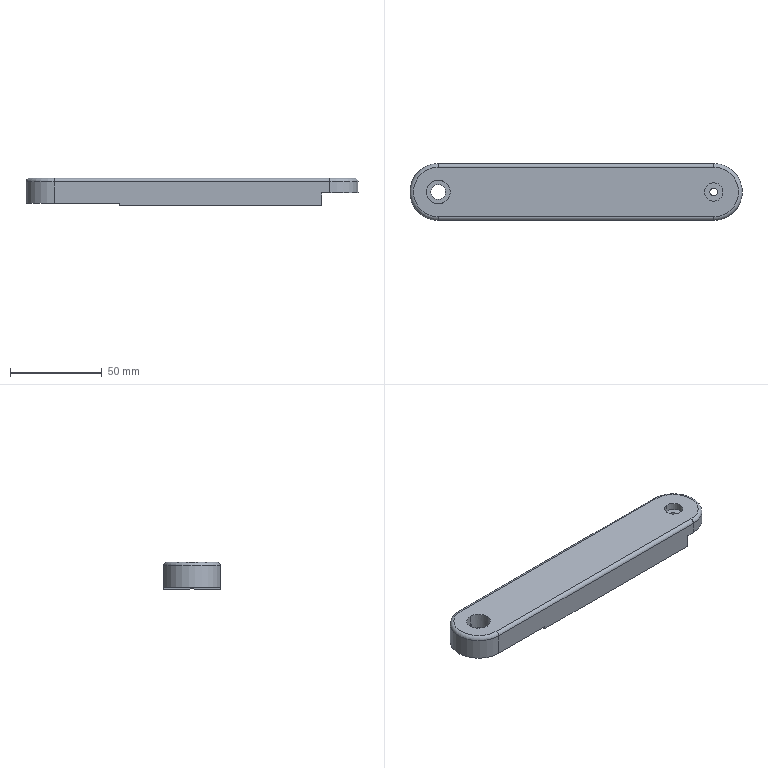NC program | NX | posted with a generic post | part box 181 x 31 x 15 mm
Lines 1657 to 2910 of 2910:
(FIXED_CONTOUR , TOOL : R2)
N3222 T21 M6
N3224 G54
N3226 G17 G0 G90 X1.241 Y-0.541 S9500 M3
N3228 G43 Z30. H21
N3230 Z3.6
N3232 G94 G1 Z-0.539 F1000.
N3234 X1.217 Y-0.511
N3236 X1.179 Y-0.512
N3238 X1.1 F2500.
N3240 X-0.1
N3242 X-1.3
N3244 X-2.5
N3246 X-3.7
N3248 X-4.9 Z-0.54
N3250 X-6.1 Y-0.511
N3252 X-7.3
N3254 X-8.5
N3256 X-9.7 Z-0.541
N3258 X-10.9
N3260 X-12.1
N3262 X-13.3 Z-0.542
N3264 X-14.5
N3266 X-15.7
N3268 X-16.9 Y-0.51 Z-0.543
N3270 X-18.1
N3272 X-19.3 Z-0.544
N3274 X-20.5
N3276 X-21.7 Z-0.545
N3278 X-22.9
N3280 X-24.1
N3282 X-25.3 Z-0.546
N3284 X-26.5 Y-0.509
N3286 X-27.7 Z-0.547
N3288 X-28.9
N3290 X-30.1 Z-0.548
N3292 X-31.3
N3294 X-32.5 Z-0.549
N3296 X-33.7
N3298 X-34.9
N3300 X-36.1 Y-0.508 Z-0.55
N3302 X-37.3
N3304 X-38.5
N3306 X-39.7
N3308 X-40.9
N3310 X-42.1
N3312 X-43.3
N3314 X-44.5 Z-0.551
N3316 X-45.7
N3318 X-46.9 Y-0.507
N3320 X-48.1
N3322 X-49.3
N3324 X-50.5
N3326 X-51.7
N3328 X-52.9
N3330 X-54.1
N3332 X-55.3 Z-0.552
N3334 X-56.5 Y-0.506
N3336 X-57.7
N3338 X-58.9
N3340 X-59.348
N3342 X-59.324 Y-0.42 Z-0.62
N3344 X-58.9
N3346 X-57.7 Z-0.619
N3348 X-56.5
N3350 X-55.3
N3352 X-54.1 Z-0.618
N3354 X-52.9 Y-0.421
N3356 X-51.7 Z-0.617
N3358 X-50.5
N3360 X-49.3 Z-0.616
N3362 X-48.1
N3364 X-46.9 Z-0.615
N3366 X-45.7
N3368 X-44.5
N3370 X-43.3 Y-0.422 Z-0.614
N3372 X-42.1
N3374 X-40.9 Z-0.613
N3376 X-39.7
N3378 X-38.5 Z-0.612
N3380 X-37.3
N3382 X-36.1
N3384 X-34.9 Z-0.611
N3386 X-33.7
N3388 X-32.5 Y-0.423
N3390 X-31.3
N3392 X-30.1 Z-0.61
N3394 X-28.9
N3396 X-27.7
N3398 X-26.5
N3400 X-25.3 Z-0.609
N3402 X-24.1
N3404 X-22.9 Y-0.424
N3406 X-21.7
N3408 X-20.5
N3410 X-19.3
N3412 X-18.1
N3414 X-16.9
N3416 X-15.7 Z-0.608
N3418 X-14.5
N3420 X-13.3
N3422 X-12.1 Y-0.425
N3424 X-10.9
N3426 X-9.7
N3428 X-8.5
N3430 X-7.3
N3432 X-6.1
N3434 X-4.9
N3436 X-3.7
N3438 X-2.5 Y-0.426 Z-0.607
N3440 X-1.3
N3442 X-0.1
N3444 X1.1
N3446 X2.3
N3448 X3.5
N3450 X4.7
N3452 X5.9
N3454 X7.1
N3456 X8.3 Y-0.427
N3458 X9.5
N3460 X10.7 Z-0.606
N3462 X11.9
N3464 X13.1
N3466 X14.3
N3468 X15.5
N3470 X16.7
N3472 X17.9 Y-0.428
N3474 X19.1
N3476 X20.3
N3478 X21.5
N3480 X22.7 Z-0.605
N3482 X23.9
N3484 X25.1
N3486 X26.3
N3488 X27.5 Y-0.429
N3490 X28.7
N3492 X29.9
N3494 X31.1
N3496 X32.3
N3498 X33.5
N3500 X34.7
N3502 X35.9 Z-0.604
N3504 X37.1
N3506 X38.3 Y-0.43
N3508 X39.5
N3510 Y-0.391 Z-0.63
N3512 Y-0.336 Z-0.66
N3514 X38.3 Y-0.335
N3516 X37.1
N3518 X35.9 Z-0.661
N3520 X34.7
N3522 X33.5
N3524 X32.3
N3526 X31.1
N3528 X29.9
N3530 X28.7
N3532 X27.5 Y-0.334
N3534 X26.3
N3536 X25.1
N3538 X23.9
N3540 X22.7
N3542 X21.5
N3544 X20.3
N3546 X19.1
N3548 X17.9 Y-0.333 Z-0.662
N3550 X16.7
N3552 X15.5
N3554 X14.3
N3556 X13.1
N3558 X11.9
N3560 X10.7
N3562 X9.5
N3564 X8.3 Y-0.332
N3566 X7.1
N3568 X5.9
N3570 X4.7
N3572 X3.5
N3574 X2.3
N3576 X1.1
N3578 X-0.1 Z-0.663
N3580 X-1.3
N3582 X-2.5 Y-0.331
N3584 X-3.7
N3586 X-4.9
N3588 X-6.1
N3590 X-7.3
N3592 X-8.5
N3594 X-9.7
N3596 X-10.9
N3598 X-12.1 Y-0.33
N3600 X-13.3
N3602 X-14.5
N3604 X-15.7
N3606 X-16.9
N3608 X-18.1
N3610 X-19.3 Z-0.664
N3612 X-20.5
N3614 X-21.7
N3616 X-22.9 Y-0.329
N3618 X-24.1
N3620 X-25.3
N3622 X-26.5 Z-0.665
N3624 X-27.7
N3626 X-28.9
N3628 X-30.1
N3630 X-31.3
N3632 X-32.5 Y-0.328 Z-0.666
N3634 X-33.7
N3636 X-34.9
N3638 X-36.1 Z-0.667
N3640 X-37.3
N3642 X-38.5
N3644 X-39.7 Z-0.668
N3646 X-40.9
N3648 X-42.1
N3650 X-43.3 Y-0.327 Z-0.669
N3652 X-44.5
N3654 X-45.7
N3656 X-46.9 Z-0.67
N3658 X-48.1
N3660 X-49.3
N3662 X-50.5 Z-0.671
N3664 X-51.7
N3666 X-52.9 Y-0.326
N3668 X-54.1
N3670 X-55.3 Z-0.672
N3672 X-56.5
N3674 X-57.7
N3676 X-58.9 Z-0.673
N3678 X-59.301
N3680 X-59.281 Y-0.232 Z-0.711
N3682 X-58.9
N3684 X-57.7
N3686 X-56.5 Z-0.71
N3688 X-55.3
N3690 X-54.1
N3692 X-52.9 Z-0.709
N3694 X-51.7
N3696 X-50.5 Y-0.233
N3698 X-49.3
N3700 X-48.1 Z-0.708
N3702 X-46.9
N3704 X-45.7
N3706 X-44.5 Z-0.707
N3708 X-43.3
N3710 X-42.1
N3712 X-40.9 Y-0.234
N3714 X-39.7 Z-0.706
N3716 X-38.5
N3718 X-37.3
N3720 X-36.1 Z-0.705
N3722 X-34.9
N3724 X-33.7
N3726 X-32.5
N3728 X-31.3 Z-0.704
N3730 X-30.1 Y-0.235
N3732 X-28.9
N3734 X-27.7
N3736 X-26.5 Z-0.703
N3738 X-25.3
N3740 X-24.1
N3742 X-22.9
N3744 X-21.7 Z-0.702
N3746 X-20.5 Y-0.236
N3748 X-19.3
N3750 X-18.1
N3752 X-16.9
N3754 X-15.7
N3756 X-14.5
N3758 X-13.3
N3760 X-12.1
N3762 X-10.9
N3764 X-9.7 Y-0.237
N3766 X-8.5 Z-0.701
N3768 X-7.3
N3770 X-6.1
N3772 X-4.9
N3774 X-3.7
N3776 X-2.5
N3778 X-1.3
N3780 X-0.1 Y-0.238
N3782 X1.1
N3784 X2.3
N3786 X3.5
N3788 X4.7
N3790 X5.9
N3792 X7.1
N3794 X8.3
N3796 X9.5
N3798 X10.7 Y-0.239
N3800 X11.9
N3802 X13.1
N3804 X14.3
N3806 X15.5
N3808 X16.7
N3810 X17.9
N3812 X19.1
N3814 X20.3 Y-0.24 Z-0.7
N3816 X21.5
N3818 X22.7
N3820 X23.9
N3822 X25.1
N3824 X26.3
N3826 X27.5
N3828 X28.7
N3830 X29.9 Y-0.241
N3832 X31.1
N3834 X32.3
N3836 X33.5
N3838 X34.7
N3840 X35.9
N3842 X37.1
N3844 X38.3
N3846 X39.5
N3848 Y-0.195 Z-0.716
N3850 Y-0.147 Z-0.726
N3852 X38.3
N3854 X37.1
N3856 X35.9
N3858 X34.7
N3860 X33.5
N3862 X32.3
N3864 X31.1
N3866 X29.9 Y-0.146
N3868 X28.7
N3870 X27.5
N3872 X26.3
N3874 X25.1
N3876 X23.9
N3878 X22.7
N3880 X21.5
N3882 X20.3 Y-0.145
N3884 X19.1
N3886 X17.9
N3888 X16.7
N3890 X15.5
N3892 X14.3
N3894 X13.1
N3896 X11.9
N3898 X10.7 Y-0.144
N3900 X9.5
N3902 X8.3
N3904 X7.1
N3906 X5.9
N3908 X4.7
N3910 X3.5
N3912 X2.3
N3914 X1.1 Z-0.727
N3916 X-0.1 Y-0.143
N3918 X-1.3
N3920 X-2.5
N3922 X-3.7
N3924 X-4.9
N3926 X-6.1
N3928 X-7.3
N3930 X-8.5
N3932 X-9.7 Y-0.142
N3934 X-10.9
N3936 X-12.1
N3938 X-13.3
N3940 X-14.5
N3942 X-15.7
N3944 X-16.9
N3946 X-18.1 Z-0.728
N3948 X-19.3
N3950 X-20.5 Y-0.141
N3952 X-21.7
N3954 X-22.9
N3956 X-24.1 Z-0.729
N3958 X-25.3
N3960 X-26.5
N3962 X-27.7 Z-0.73
N3964 X-28.9
N3966 X-30.1 Y-0.14
N3968 X-31.3
N3970 X-32.5 Z-0.731
N3972 X-33.7
N3974 X-34.9
N3976 X-36.1 Z-0.732
N3978 X-37.3
N3980 X-38.5
N3982 X-39.7 Z-0.733
N3984 X-40.9 Y-0.139
N3986 X-42.1
N3988 X-43.3 Z-0.734
N3990 X-44.5
N3992 X-45.7
N3994 X-46.9 Z-0.735
N3996 X-48.1
N3998 X-49.3
N4000 X-50.5 Y-0.138
N4002 X-51.7
N4004 X-52.9 Z-0.736
N4006 X-54.1
N4008 X-55.3
N4010 X-56.5
N4012 X-57.7
N4014 X-58.9
N4016 X-59.269
N4018 X-59.261 Y-0.043 Z-0.746
N4020 X-58.9 Y-0.044
N4022 X-57.7
N4024 X-56.5
N4026 X-55.3
N4028 X-54.1
N4030 X-52.9
N4032 X-51.7
N4034 X-50.5
N4036 X-49.3
N4038 X-48.1 Y-0.045
N4040 X-46.9 Z-0.745
N4042 X-45.7
N4044 X-44.5
N4046 X-43.3
N4048 X-42.1 Z-0.744
N4050 X-40.9
N4052 X-39.7
N4054 X-38.5 Y-0.046
N4056 X-37.3
N4058 X-36.1
N4060 X-34.9 Z-0.743
N4062 X-33.7
N4064 X-32.5
N4066 X-31.3
N4068 X-30.1
N4070 X-28.9
N4072 X-27.7 Y-0.047
N4074 X-26.5
N4076 X-25.3
N4078 X-24.1
N4080 X-22.9
N4082 X-21.7
N4084 X-20.5
N4086 X-19.3
N4088 X-18.1 Y-0.048
N4090 X-16.9
N4092 X-15.7
N4094 X-14.5
N4096 X-13.3
N4098 X-12.1
N4100 X-10.9
N4102 X-9.7
N4104 X-8.5
N4106 X-7.3 Y-0.049
N4108 X-6.1
N4110 X-4.9
N4112 X-3.7
N4114 X-2.5
N4116 X-1.3
N4118 X-0.1
N4120 X1.1 Z-0.742
N4122 X2.3 Y-0.05
N4124 X3.5
N4126 X4.7
N4128 X5.9
N4130 X7.1
N4132 X8.3
N4134 X9.5
N4136 X10.7
N4138 X11.9
N4140 X13.1 Y-0.051
N4142 X14.3
N4144 X15.5
N4146 X16.7
N4148 X17.9
N4150 X19.1
N4152 X20.3
N4154 X21.5
N4156 X22.7 Y-0.052
N4158 X23.9
N4160 X25.1
N4162 X26.3
N4164 X27.5
N4166 X28.7
N4168 X29.9
N4170 X31.1
N4172 X32.3 Y-0.053
N4174 X33.5
N4176 X34.7
N4178 X35.9
N4180 X37.1
N4182 X38.3
N4184 X39.5
N4186 Y0. Z-0.748
N4188 Y0.041 Z-0.744
N4190 X38.3
N4192 X37.1
N4194 X35.9
N4196 X34.7
N4198 X33.5
N4200 X32.3 Y0.042
N4202 X31.1 Z-0.745
N4204 X29.9
N4206 X28.7
N4208 X27.5
N4210 X26.3
N4212 X25.1
N4214 X23.9
N4216 X22.7 Y0.043
N4218 X21.5
N4220 X20.3
N4222 X19.1
N4224 X17.9
N4226 X16.7
N4228 X15.5 Z-0.746
N4230 X14.3
N4232 X13.1 Y0.044
N4234 X11.9
N4236 X10.7
N4238 X9.5
N4240 X8.3
N4242 X7.1
N4244 X5.9
N4246 X4.7
N4248 X3.5
N4250 X2.3 Y0.045
N4252 X1.1
N4254 X-0.1
N4256 X-1.3
N4258 X-2.5
N4260 X-3.7
N4262 X-4.9
N4264 X-6.1
N4266 X-7.3 Y0.046
N4268 X-8.5
N4270 X-9.7
N4272 X-10.9
N4274 X-12.1
N4276 X-13.3
N4278 X-14.5
N4280 X-15.7
N4282 X-16.9
N4284 X-18.1 Y0.047
N4286 X-19.3
N4288 X-20.5
N4290 X-21.7
N4292 X-22.9
N4294 X-24.1
N4296 X-25.3
N4298 X-26.5
N4300 X-27.7 Y0.048
N4302 X-28.9
N4304 X-30.1
N4306 X-31.3
N4308 X-32.5
N4310 X-33.7
N4312 X-34.9
N4314 X-36.1
N4316 X-37.3
N4318 X-38.5 Y0.049
N4320 X-39.7
N4322 X-40.9
N4324 X-42.1
N4326 X-43.3
N4328 X-44.5
N4330 X-45.7
N4332 X-46.9
N4334 X-48.1 Y0.05
N4336 X-49.3
N4338 X-50.5
N4340 X-51.7
N4342 X-52.9
N4344 X-54.1
N4346 X-55.3
N4348 X-56.5
N4350 X-57.7
N4352 X-58.9 Y0.051
N4354 X-59.262
N4356 X-59.269 Y0.145 Z-0.735
N4358 X-58.9
N4360 X-57.7
N4362 X-56.5 Y0.144
N4364 X-55.3
N4366 X-54.1
N4368 X-52.9 Z-0.734
N4370 X-51.7
N4372 X-50.5
N4374 X-49.3
N4376 X-48.1
N4378 X-46.9
N4380 X-45.7 Y0.143
N4382 X-44.5
N4384 X-43.3
N4386 X-42.1
N4388 X-40.9 Z-0.733
N4390 X-39.7
N4392 X-38.5
N4394 X-37.3
N4396 X-36.1 Y0.142
N4398 X-34.9
N4400 X-33.7
N4402 X-32.5
N4404 X-31.3
N4406 X-30.1
N4408 X-28.9
N4410 X-27.7
N4412 X-26.5 Z-0.732
N4414 X-25.3 Y0.141
N4416 X-24.1
N4418 X-22.9
N4420 X-21.7
N4422 X-20.5
N4424 X-19.3
N4426 X-18.1
N4428 X-16.9
N4430 X-15.7 Y0.14
N4432 X-14.5
N4434 X-13.3
N4436 X-12.1
N4438 X-10.9 Z-0.731
N4440 X-9.7
N4442 X-8.5
N4444 X-7.3
N4446 X-6.1
N4448 X-4.9 Y0.139
N4450 X-3.7
N4452 X-2.5
N4454 X-1.3
N4456 X-0.1
N4458 X1.1
N4460 X2.3
N4462 X3.5 Z-0.73
N4464 X4.7 Y0.138
N4466 X5.9
N4468 X7.1
N4470 X8.3
N4472 X9.5
N4474 X10.7
N4476 X11.9
N4478 X13.1
N4480 X14.3
N4482 X15.5 Y0.137
N4484 X16.7
N4486 X17.9 Z-0.729
N4488 X19.1
N4490 X20.3
N4492 X21.5
N4494 X22.7
N4496 X23.9
N4498 X25.1 Y0.136
N4500 X26.3
N4502 X27.5
N4504 X28.7
N4506 X29.9
N4508 X31.1
N4510 X32.3 Z-0.728
N4512 X33.5
N4514 X34.7 Y0.135
N4516 X35.9
N4518 X37.1
N4520 X38.3
N4522 X39.5
N4524 Y0.195 Z-0.716
N4526 Y0.229 Z-0.704
N4528 X38.3
N4530 X37.1
N4532 X35.9
N4534 X34.7 Y0.23
N4536 X33.5 Z-0.705
N4538 X32.3
N4540 X31.1
N4542 X29.9
N4544 X28.7
N4546 X27.5
N4548 X26.3
N4550 X25.1 Y0.231
N4552 X23.9
N4554 X22.7
N4556 X21.5
N4558 X20.3
N4560 X19.1 Z-0.706
N4562 X17.9
N4564 X16.7
N4566 X15.5 Y0.232
N4568 X14.3
N4570 X13.1
N4572 X11.9
N4574 X10.7
N4576 X9.5
N4578 X8.3
N4580 X7.1
N4582 X5.9
N4584 X4.7 Y0.233 Z-0.707
N4586 X3.5
N4588 X2.3
N4590 X1.1
N4592 X-0.1
N4594 X-1.3
N4596 X-2.5
N4598 X-3.7
N4600 X-4.9 Y0.234
N4602 X-6.1
N4604 X-7.3
N4606 X-8.5
N4608 X-9.7 Z-0.708
N4610 X-10.9
N4612 X-12.1
N4614 X-13.3
N4616 X-14.5
N4618 X-15.7 Y0.235
N4620 X-16.9
N4622 X-18.1
N4624 X-19.3
N4626 X-20.5
N4628 X-21.7
N4630 X-22.9
N4632 X-24.1 Z-0.709
N4634 X-25.3 Y0.236
N4636 X-26.5
N4638 X-27.7
N4640 X-28.9
N4642 X-30.1
N4644 X-31.3
N4646 X-32.5
N4648 X-33.7
N4650 X-34.9
N4652 X-36.1 Y0.237
N4654 X-37.3
N4656 X-38.5
N4658 X-39.7
N4660 X-40.9
N4662 X-42.1
N4664 X-43.3
N4666 X-44.5
N4668 X-45.7 Y0.238
N4670 X-46.9
N4672 X-48.1
N4674 X-49.3
N4676 X-50.5
N4678 X-51.7
N4680 X-52.9
N4682 X-54.1
N4684 X-55.3
N4686 X-56.5 Y0.239
N4688 X-57.7
N4690 X-58.9
N4692 X-59.283
N4694 X-59.303 Y0.333 Z-0.669
N4696 X-58.9
N4698 X-57.7
N4700 X-56.5
N4702 X-55.3 Z-0.67
N4704 X-54.1 Y0.332
N4706 X-52.9
N4708 X-51.7
N4710 X-50.5
N4712 X-49.3
N4714 X-48.1
N4716 X-46.9
N4718 X-45.7
N4720 X-44.5
N4722 X-43.3 Y0.331
N4724 X-42.1
N4726 X-40.9
N4728 X-39.7
N4730 X-38.5
N4732 X-37.3
N4734 X-36.1
N4736 X-34.9 Z-0.671
N4738 X-33.7 Y0.33
N4740 X-32.5
N4742 X-31.3
N4744 X-30.1
N4746 X-28.9
N4748 X-27.7
N4750 X-26.5
N4752 X-25.3
N4754 X-24.1
N4756 X-22.9 Y0.329
N4758 X-21.7
N4760 X-20.5
N4762 X-19.3
N4764 X-18.1 Z-0.67
N4766 X-16.9
N4768 X-15.7
N4770 X-14.5
N4772 X-13.3 Y0.328
N4774 X-12.1
N4776 X-10.9
N4778 X-9.7
N4780 X-8.5
N4782 X-7.3
N4784 X-6.1
N4786 X-4.9
N4788 X-3.7
N4790 X-2.5 Y0.327
N4792 X-1.3
N4794 X-0.1 Z-0.669
N4796 X1.1
N4798 X2.3
N4800 X3.5
N4802 X4.7
N4804 X5.9
N4806 X7.1 Y0.326
N4808 X8.3
N4810 X9.5
N4812 X10.7
N4814 X11.9
N4816 X13.1
N4818 X14.3
N4820 X15.5
N4822 X16.7 Z-0.668
N4824 X17.9 Y0.325
N4826 X19.1
N4828 X20.3
N4830 X21.5
N4832 X22.7
N4834 X23.9
N4836 X25.1
N4838 X26.3
N4840 X27.5 Y0.324
N4842 X28.7
N4844 X29.9
N4846 X31.1
N4848 X32.3
N4850 X33.5 Z-0.667
N4852 X34.7
N4854 X35.9
N4856 X37.1 Y0.323
N4858 X38.3
N4860 X39.5
N4862 Y0.417 Z-0.614
N4864 X38.3
N4866 X37.1 Y0.418
N4868 X35.9
N4870 X34.7
N4872 X33.5
N4874 X32.3
N4876 X31.1
N4878 X29.9
N4880 X28.7
N4882 X27.5 Y0.419
N4884 X26.3
N4886 X25.1
N4888 X23.9 Z-0.615
N4890 X22.7
N4892 X21.5
N4894 X20.3
N4896 X19.1
N4898 X17.9 Y0.42
N4900 X16.7
N4902 X15.5
N4904 X14.3
N4906 X13.1
N4908 X11.9
N4910 X10.7
N4912 X9.5
N4914 X8.3
N4916 X7.1 Y0.421
N4918 X5.9
N4920 X4.7
N4922 X3.5
N4924 X2.3
N4926 X1.1
N4928 X-0.1
N4930 X-1.3
N4932 X-2.5 Y0.422
N4934 X-3.7 Z-0.616
N4936 X-4.9
N4938 X-6.1
N4940 X-7.3
N4942 X-8.5
N4944 X-9.7
N4946 X-10.9
N4948 X-12.1
N4950 X-13.3 Y0.423
N4952 X-14.5
N4954 X-15.7
N4956 X-16.9
N4958 X-18.1
N4960 X-19.3
N4962 X-20.5
N4964 X-21.7
N4966 X-22.9 Y0.424
N4968 X-24.1
N4970 X-25.3
N4972 X-26.5
N4974 X-27.7
N4976 X-28.9
N4978 X-30.1
N4980 X-31.3
N4982 X-32.5
N4984 X-33.7 Y0.425
N4986 X-34.9
N4988 X-36.1
N4990 X-37.3
N4992 X-38.5
N4994 X-39.7
N4996 X-40.9
N4998 X-42.1
N5000 X-43.3 Y0.426
N5002 X-44.5
N5004 X-45.7
N5006 X-46.9
N5008 X-48.1
N5010 X-49.3
N5012 X-50.5
N5014 X-51.7
N5016 X-52.9
N5018 X-54.1 Y0.427
N5020 X-55.3 Z-0.615
N5022 X-56.5
N5024 X-57.7
N5026 X-58.9
N5028 X-59.326
N5030 X-59.35 Y0.514 Z-0.545
N5032 X-58.9
N5034 X-57.7
N5036 X-56.5
N5038 X-55.3
N5040 X-54.1
N5042 X-52.9
N5044 X-51.7 Y0.513
N5046 X-50.5 Z-0.546
N5048 X-49.3
N5050 X-48.1
N5052 X-46.9
N5054 X-45.7
N5056 X-44.5
N5058 X-43.3
N5060 X-42.1 Y0.512
N5062 X-40.9
N5064 X-39.7 Z-0.547
N5066 X-38.5
N5068 X-37.3
N5070 X-36.1
N5072 X-34.9
N5074 X-33.7
N5076 X-32.5
N5078 X-31.3 Y0.511
N5080 X-30.1
N5082 X-28.9
N5084 X-27.7
N5086 X-26.5
N5088 X-25.3
N5090 X-24.1
N5092 X-22.9
N5094 X-21.7 Y0.51
N5096 X-20.5
N5098 X-19.3
N5100 X-18.1
N5102 X-16.9
N5104 X-15.7
N5106 X-14.5
N5108 X-13.3
N5110 X-12.1
N5112 X-10.9 Y0.509 Z-0.546
N5114 X-9.7
N5116 X-8.5
N5118 X-7.3
N5120 X-6.1
N5122 X-4.9
N5124 X-3.7
N5126 X-2.5
N5128 X-1.3 Y0.508
N5130 X-0.1
N5132 X1.1
N5134 X2.3
N5136 X3.5
N5138 X4.7
N5140 X5.9
N5142 X7.1
N5144 X8.3
N5146 X9.5 Y0.507
N5148 X10.7
N5150 X11.9
N5152 X13.1
N5154 X14.3
N5156 X15.5
N5158 X16.7 Z-0.545
N5160 X17.9
N5162 X19.1 Y0.506
N5164 X20.3
N5166 X21.5
N5168 X22.7
N5170 X23.9
N5172 X25.1
N5174 X26.3
N5176 X27.5
N5178 X28.7
N5180 X29.9 Y0.505
N5182 X31.1
N5184 X32.3
N5186 X33.5
N5188 X34.7
N5190 X35.9
N5192 X37.1
N5194 X38.3
N5196 X39.5 Y0.504
N5198 G2 X39.806 Y0.362 R0.4
N5200 G1 Z2.8
N5202 G0 Z30.
N5204 M5
(PLANAR_MILL_COPY_COPY_COPY_COPY_COPY_COPY_1_COPY_1 , TOOL : D6A45)
N5206 T01 M6
N5208 G54
N5210 G17 G0 G90 X41.762 Y-3.361 S9500 M3
N5212 G43 Z30. H1
N5214 Z0.5
N5216 G94 G1 Z-1. F1250.
N5218 X41.299 Y-3.117
N5220 G3 X40.3 Y-3.156 R1.
N5222 G1 Y-15.3
N5224 G2 X39.3 Y-16.3 R1.
N5226 G1 X-70.493
N5228 G2 X-70.776 Y-14.341 R1.
N5230 G3 X-60.357 Y-3.012 R14.95
N5232 X-61.337 Y-2.813 R1.
N5234 G1 Y2.813
N5236 G3 X-60.357 Y3.012 R1.
N5238 X-70.776 Y14.341 R14.95
N5240 G2 X-70.493 Y16.3 R1.
N5242 G1 X39.3
N5244 G2 X40.3 Y15.3 R1.
N5246 G1 Y3.156
N5248 G3 X41.299 Y3.117 R1.
N5250 G1 X41.762 Y3.361
N5252 Z0.5
N5254 G0 Z30.
(PLANAR_MILL_COPY_COPY_COPY_COPY_COPY_COPY_1_COPY_1_COPY , TOOL : D6A45)
N5256 X-79.648 Y7.597
N5258 Z-6.5
N5260 G1 X-79.38 Y7.569 Z-6.575
N5262 X-79.275 Y7.674 Z-6.615
N5264 Y7.914 Z-6.679
N5266 X-79.38 Y8.019 Z-6.719
N5268 X-79.62 Z-6.783
N5270 X-79.725 Y7.914 Z-6.823
N5272 Y7.674 Z-6.887
N5274 X-79.62 Y7.569 Z-6.927
N5276 X-79.38 Z-6.991
N5278 X-79.275 Y7.674 Z-7.031
N5280 Y7.914 Z-7.095
N5282 X-79.38 Y8.019 Z-7.135
N5284 X-79.62 Z-7.199
N5286 X-79.725 Y7.914 Z-7.239
N5288 Y7.674 Z-7.303
N5290 X-79.62 Y7.569 Z-7.343
N5292 X-79.38 Z-7.408
N5294 X-79.275 Y7.674 Z-7.447
N5296 Y7.914 Z-7.512
N5298 X-79.38 Y8.019 Z-7.551
N5300 X-79.62 Z-7.616
N5302 X-79.725 Y7.914 Z-7.656
N5304 Y7.674 Z-7.72
N5306 X-79.62 Y7.569 Z-7.76
N5308 X-79.38 Z-7.824
N5310 X-79.275 Y7.674 Z-7.864
N5312 Y7.914 Z-7.928
N5314 X-79.38 Y8.019 Z-7.968
N5316 X-79.5 Z-8.
N5318 G3 X-79.725 Y7.794 R0.225
N5320 X-79.5 Y8.019 R-0.225
N5322 X-79.538 Y7.763 R0.5
N5324 G1 Z-6.5
N5326 G0 Z30.
N5328 X-75.068 Y0.073
N5330 Z-6.5
N5332 G1 Z-8.
N5334 X-75.8 Y0.866
N5336 G3 X-76.3 Y0. R1.
N5338 X-75. Y-1.3 R1.3
N5340 X-76.3 Y0. R-1.3
N5342 X-75.8 Y-0.866 R1.
N5344 G1 X-75.068 Y-0.073
N5346 Z-6.5
N5348 G0 Z30.
N5350 X-70.352 Y-7.597
N5352 Z-6.5
N5354 G1 X-70.62 Y-7.569 Z-6.575
N5356 X-70.725 Y-7.674 Z-6.615
N5358 Y-7.914 Z-6.679
N5360 X-70.62 Y-8.019 Z-6.719
N5362 X-70.38 Z-6.783
N5364 X-70.275 Y-7.914 Z-6.823
N5366 Y-7.674 Z-6.887
N5368 X-70.38 Y-7.569 Z-6.927
N5370 X-70.62 Z-6.991
N5372 X-70.725 Y-7.674 Z-7.031
N5374 Y-7.914 Z-7.095
N5376 X-70.62 Y-8.019 Z-7.135
N5378 X-70.38 Z-7.199
N5380 X-70.275 Y-7.914 Z-7.239
N5382 Y-7.674 Z-7.303
N5384 X-70.38 Y-7.569 Z-7.343
N5386 X-70.62 Z-7.408
N5388 X-70.725 Y-7.674 Z-7.447
N5390 Y-7.914 Z-7.512
N5392 X-70.62 Y-8.019 Z-7.551
N5394 X-70.38 Z-7.616
N5396 X-70.275 Y-7.914 Z-7.656
N5398 Y-7.674 Z-7.72
N5400 X-70.38 Y-7.569 Z-7.76
N5402 X-70.62 Z-7.824
N5404 X-70.725 Y-7.674 Z-7.864
N5406 Y-7.914 Z-7.928
N5408 X-70.62 Y-8.019 Z-7.968
N5410 X-70.5 Z-8.
N5412 G3 X-70.275 Y-7.794 R0.225
N5414 X-70.5 Y-8.019 R-0.225
N5416 X-70.462 Y-7.763 R0.5
N5418 G1 Z-6.5
N5420 G0 Z30.
N5422 X-74.75 Y-17.727
N5424 Z-6.5
N5426 G1 Z-8.
N5428 X-74.303 Y-17.269
N5430 G3 X-74.055 Y-16.3 R1.
N5432 G1 X-75.
N5434 G2 X-91.3 Y0. R16.3
N5436 X-75. Y16.3 R16.3
N5438 G1 X-74.055
N5440 G3 X-74.303 Y17.269 R1.
N5442 G1 X-74.75 Y17.727
N5444 Z-6.5
N5446 G0 Z30.
(PLANAR_MILL_COPY_COPY_COPY_COPY_COPY_COPY_1_COPY_1_COPY_COPY , TOOL : D6A45)
N5448 X42.832 Y17.713
N5450 Z-0.8
N5452 G1 Z-2.3
N5454 X42.415 Y17.273
N5456 G3 X42.183 Y16.3 R1.
N5458 G1 X75.
N5460 G2 X91.3 Y0. R16.3
N5462 X75. Y-16.3 R16.3
N5464 G1 X42.183
N5466 G3 X42.415 Y-17.273 R1.
N5468 G1 X42.832 Y-17.713
N5470 Z-0.8
N5472 G0 Z30.
N5474 X43.5 Y-7.93
N5476 Z-0.8
N5478 G1 Z-2.3
N5480 X42.8 Y-8.334
N5482 G3 X42.3 Y-9.2 R1.
N5484 G1 X62.5
N5486 G2 X64.3 Y-11. R1.8
N5488 G1 Y-13.8
N5490 G3 X64.5 Y-14. R0.2
N5492 G1 X75.
N5494 G3 X78.5 Y-10.5 R3.5
N5496 X75. Y-7. R3.5
N5498 G1 X70.5
N5500 G2 X68.7 Y-5.2 R1.8
N5502 G1 Y5.2
N5504 G2 X70.5 Y7. R1.8
N5506 G1 X75.
N5508 G3 X78.5 Y10.5 R3.5
N5510 X75. Y14. R3.5
N5512 G1 X64.5
N5514 G3 X64.3 Y13.8 R0.2
N5516 G1 Y11.
N5518 G2 X62.5 Y9.2 R1.8
N5520 G1 X42.3
N5522 G3 X42.8 Y8.334 R1.
N5524 G1 X43.5 Y7.93
N5526 Z-0.8
N5528 G0 Z30.
N5530 X76.904 Y-0.611
N5532 Z-0.8
N5534 G1 Z-2.3
N5536 X77.7 Y-0.866
N5538 G3 X78.2 Y0. R1.
N5540 X75. Y3.2 R3.2
N5542 X78.2 Y0. R-3.2
N5544 X77.7 Y0.866 R1.
N5546 G1 X76.904 Y0.611
N5548 Z-0.8
N5550 G0 Z30.
(DRILLING_COPY_1_COPY_2 , TOOL : D6A45)
N5552 X-79.5 Y7.794 S5000
N5554 G81 G98 Z-8.05 F350. R-4.
N5556 X-75. Y0.
N5558 X-70.5 Y-7.794
N5560 X43. Y-12.5 Z-2.35 R1.7
N5562 X61.
N5564 Y12.5
N5566 X43.
N5568 G80
N5570 G0 X43. Y12.5 Z30.
N5572 M5
(刀补11 , TOOL : D4)
N5574 T11 M6
N5576 G54
N5578 G17 G0 G90 X75. Y0. S9500 M3
N5580 G43 Z30. H11
N5582 Z-0.8
N5584 G41 G94 G1 X75.007 Y0.1 F1000. D11
N5586 G3 X73.05 Y0. R0.981
N5588 X73.05 Y0. Z-2.8 I1.95 J0.
N5590 X73.05 Y0. Z-4.8 I1.95 J0.
N5592 X73.05 Y0. Z-6.8 I1.95 J0.
N5594 X73.05 Y0. Z-8.8 I1.95 J0.
N5596 X73.05 Y0. Z-10.8 I1.95 J0.
N5598 X73.05 Y0. Z-12.8 I1.95 J0.
N5600 X73.05 Y0. Z-14.8 I1.95 J0.
N5602 X73.422 Y-1.146 Z-15. R1.95
N5604 X76.146 Y-1.578 R1.95
N5606 X73.422 Y-1.146 R-1.95
N5608 X75.065 Y-0.076 R0.981
N5610 G40
N5612 G1 X75. Y0.
N5614 G0 Z30.
N5616 M5
(刀补12 , TOOL : D6)
N5618 T12 M6
N5620 G54
N5622 G17 G0 G90 X75. Y10.5 S9500 M3
N5624 G43 Z30. H12
N5626 Z-0.8
N5628 G41 G94 G1 X75.002 Y10.6 F1000. D12
N5630 G3 X73.75 Y10.5 R0.63
N5632 X73.75 Y10.5 Z-2.8 I1.25 J0.
N5634 X73.75 Y10.5 Z-4.8 I1.25 J0.
N5636 X73.75 Y10.5 Z-6.8 I1.25 J0.
N5638 X73.75 Y10.5 Z-8.8 I1.25 J0.
N5640 X73.989 Y9.765 Z-9. R1.25
N5642 X75.735 Y9.489 R1.25
N5644 X73.989 Y9.765 R-1.25
N5646 X75.06 Y10.42 R0.63
N5648 G40
N5650 G1 X75. Y10.5
N5652 G0 Z30.
N5654 Y-10.5
N5656 Z-0.8
N5658 G41 G1 X75.002 Y-10.4
N5660 G3 X73.75 Y-10.5 R0.63
N5662 X73.75 Y-10.5 Z-2.8 I1.25 J0.
N5664 X73.75 Y-10.5 Z-4.8 I1.25 J0.
N5666 X73.75 Y-10.5 Z-6.8 I1.25 J0.
N5668 X73.75 Y-10.5 Z-8.8 I1.25 J0.
N5670 X73.989 Y-11.235 Z-9. R1.25
N5672 X75.735 Y-11.511 R1.25
N5674 X73.989 Y-11.235 R-1.25
N5676 X75.06 Y-10.58 R0.63
N5678 G40
N5680 G1 X75. Y-10.5
N5682 G0 Z30.
N5684 M5
N5686 M2